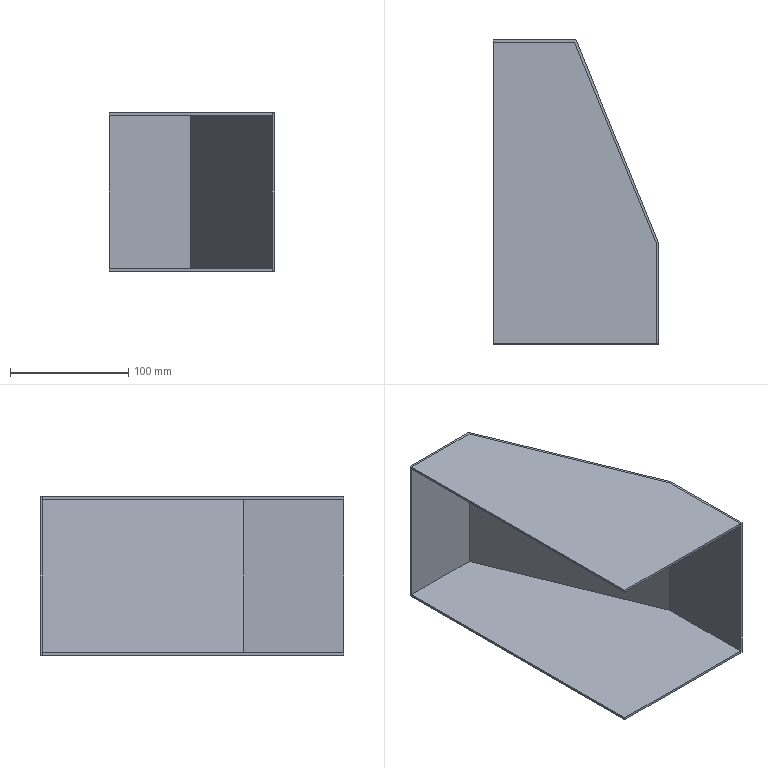Part | SolidWorks | features ICE 2, ExtruThin 1, WeldmentFeature 1 | 3 solids | 24 faces | box 140 x 257 x 134 mm | volume 207970 mm3 | plane 24
STEP:
#1=CARTESIAN_POINT('',(138.,-172.391,0.));
#2=VERTEX_POINT('',#1);
#3=CARTESIAN_POINT('',(138.,-257.,0.));
#4=VERTEX_POINT('',#3);
#5=CARTESIAN_POINT('',(138.,-172.,0.));
#6=DIRECTION('',(0.,-1.,0.));
#7=VECTOR('',#6,1000.);
#8=LINE('',#5,#7);
#9=EDGE_CURVE('',#2,#4,#8,.T.);
#10=ORIENTED_EDGE('',*,*,#9,.T.);
#11=CARTESIAN_POINT('',(138.,-257.,134.));
#12=VERTEX_POINT('',#11);
#13=CARTESIAN_POINT('',(138.,-257.,134.));
#14=DIRECTION('',(0.,0.,-1.));
#15=VECTOR('',#14,1000.);
#16=LINE('',#13,#15);
#17=EDGE_CURVE('',#12,#4,#16,.T.);
#18=ORIENTED_EDGE('',*,*,#17,.F.);
#19=CARTESIAN_POINT('',(138.,-172.391,134.));
#20=VERTEX_POINT('',#19);
#21=CARTESIAN_POINT('',(138.,-172.,134.));
#22=DIRECTION('',(0.,-1.,0.));
#23=VECTOR('',#22,1000.);
#24=LINE('',#21,#23);
#25=EDGE_CURVE('',#20,#12,#24,.T.);
#26=ORIENTED_EDGE('',*,*,#25,.F.);
#27=CARTESIAN_POINT('',(138.,-172.391,134.));
#28=DIRECTION('',(0.,0.,-1.));
#29=VECTOR('',#28,1000.);
#30=LINE('',#27,#29);
#31=EDGE_CURVE('',#20,#2,#30,.T.);
#32=ORIENTED_EDGE('',*,*,#31,.T.);
#33=EDGE_LOOP('',(#10,#18,#26,#32));
#34=FACE_OUTER_BOUND('',#33,.T.);
#35=CARTESIAN_POINT('',(138.,-172.,134.));
#36=DIRECTION('',(1.,0.,0.));
#37=DIRECTION('',(0.,1.,0.));
#38=AXIS2_PLACEMENT_3D('',#35,#36,#37);
#39=PLANE('',#38);
#40=ADVANCED_FACE('',(#34),#39,.F.);
#41=CARTESIAN_POINT('',(140.,-257.,0.));
#42=VERTEX_POINT('',#41);
#43=CARTESIAN_POINT('',(140.,-257.,0.));
#44=DIRECTION('',(-1.,0.,0.));
#45=VECTOR('',#44,1000.);
#46=LINE('',#43,#45);
#47=EDGE_CURVE('',#42,#4,#46,.T.);
#48=ORIENTED_EDGE('',*,*,#47,.F.);
#49=CARTESIAN_POINT('',(140.,-257.,134.));
#50=VERTEX_POINT('',#49);
#51=CARTESIAN_POINT('',(140.,-257.,134.));
#52=DIRECTION('',(0.,0.,-1.));
#53=VECTOR('',#52,1000.);
#54=LINE('',#51,#53);
#55=EDGE_CURVE('',#50,#42,#54,.T.);
#56=ORIENTED_EDGE('',*,*,#55,.F.);
#57=CARTESIAN_POINT('',(140.,-257.,134.));
#58=DIRECTION('',(-1.,0.,0.));
#59=VECTOR('',#58,1000.);
#60=LINE('',#57,#59);
#61=EDGE_CURVE('',#50,#12,#60,.T.);
#62=ORIENTED_EDGE('',*,*,#61,.T.);
#63=ORIENTED_EDGE('',*,*,#17,.T.);
#64=EDGE_LOOP('',(#48,#56,#62,#63));
#65=FACE_OUTER_BOUND('',#64,.T.);
#66=CARTESIAN_POINT('',(140.,-257.,134.));
#67=DIRECTION('',(0.,-1.,0.));
#68=DIRECTION('',(0.,0.,-1.));
#69=AXIS2_PLACEMENT_3D('',#66,#67,#68);
#70=PLANE('',#69);
#71=ADVANCED_FACE('',(#65),#70,.T.);
#72=CARTESIAN_POINT('',(140.,-172.,0.));
#73=VERTEX_POINT('',#72);
#74=CARTESIAN_POINT('',(140.,-172.,0.));
#75=DIRECTION('',(0.,-1.,0.));
#76=VECTOR('',#75,1000.);
#77=LINE('',#74,#76);
#78=EDGE_CURVE('',#73,#42,#77,.T.);
#79=ORIENTED_EDGE('',*,*,#78,.F.);
#80=CARTESIAN_POINT('',(140.,-172.,134.));
#81=VERTEX_POINT('',#80);
#82=CARTESIAN_POINT('',(140.,-172.,134.));
#83=DIRECTION('',(0.,0.,-1.));
#84=VECTOR('',#83,1000.);
#85=LINE('',#82,#84);
#86=EDGE_CURVE('',#81,#73,#85,.T.);
#87=ORIENTED_EDGE('',*,*,#86,.F.);
#88=CARTESIAN_POINT('',(140.,-172.,134.));
#89=DIRECTION('',(0.,-1.,0.));
#90=VECTOR('',#89,1000.);
#91=LINE('',#88,#90);
#92=EDGE_CURVE('',#81,#50,#91,.T.);
#93=ORIENTED_EDGE('',*,*,#92,.T.);
#94=ORIENTED_EDGE('',*,*,#55,.T.);
#95=EDGE_LOOP('',(#79,#87,#93,#94));
#96=FACE_OUTER_BOUND('',#95,.T.);
#97=CARTESIAN_POINT('',(140.,-172.,134.));
#98=DIRECTION('',(1.,0.,0.));
#99=DIRECTION('',(0.,1.,0.));
#100=AXIS2_PLACEMENT_3D('',#97,#98,#99);
#101=PLANE('',#100);
#102=ADVANCED_FACE('',(#96),#101,.T.);
#103=CARTESIAN_POINT('',(70.,0.,0.));
#104=VERTEX_POINT('',#103);
#105=CARTESIAN_POINT('',(70.,0.,0.));
#106=DIRECTION('',(0.377,-0.9262,0.));
#107=VECTOR('',#106,1000.);
#108=LINE('',#105,#107);
#109=EDGE_CURVE('',#104,#73,#108,.T.);
#110=ORIENTED_EDGE('',*,*,#109,.F.);
#111=CARTESIAN_POINT('',(70.,0.,134.));
#112=VERTEX_POINT('',#111);
#113=CARTESIAN_POINT('',(70.,0.,134.));
#114=DIRECTION('',(0.,0.,-1.));
#115=VECTOR('',#114,1000.);
#116=LINE('',#113,#115);
#117=EDGE_CURVE('',#112,#104,#116,.T.);
#118=ORIENTED_EDGE('',*,*,#117,.F.);
#119=CARTESIAN_POINT('',(70.,0.,134.));
#120=DIRECTION('',(0.377,-0.9262,0.));
#121=VECTOR('',#120,1000.);
#122=LINE('',#119,#121);
#123=EDGE_CURVE('',#112,#81,#122,.T.);
#124=ORIENTED_EDGE('',*,*,#123,.T.);
#125=ORIENTED_EDGE('',*,*,#86,.T.);
#126=EDGE_LOOP('',(#110,#118,#124,#125));
#127=FACE_OUTER_BOUND('',#126,.T.);
#128=CARTESIAN_POINT('',(70.,0.,134.));
#129=DIRECTION('',(0.9262,0.377,0.));
#130=DIRECTION('',(-0.377,0.9262,0.));
#131=AXIS2_PLACEMENT_3D('',#128,#129,#130);
#132=PLANE('',#131);
#133=ADVANCED_FACE('',(#127),#132,.T.);
#134=CARTESIAN_POINT('',(0.,0.,0.));
#135=VERTEX_POINT('',#134);
#136=CARTESIAN_POINT('',(0.,0.,0.));
#137=DIRECTION('',(1.,0.,0.));
#138=VECTOR('',#137,1000.);
#139=LINE('',#136,#138);
#140=EDGE_CURVE('',#135,#104,#139,.T.);
#141=ORIENTED_EDGE('',*,*,#140,.F.);
#142=CARTESIAN_POINT('',(0.,0.,134.));
#143=VERTEX_POINT('',#142);
#144=CARTESIAN_POINT('',(0.,0.,134.));
#145=DIRECTION('',(0.,0.,-1.));
#146=VECTOR('',#145,1000.);
#147=LINE('',#144,#146);
#148=EDGE_CURVE('',#143,#135,#147,.T.);
#149=ORIENTED_EDGE('',*,*,#148,.F.);
#150=CARTESIAN_POINT('',(0.,0.,134.));
#151=DIRECTION('',(1.,0.,0.));
#152=VECTOR('',#151,1000.);
#153=LINE('',#150,#152);
#154=EDGE_CURVE('',#143,#112,#153,.T.);
#155=ORIENTED_EDGE('',*,*,#154,.T.);
#156=ORIENTED_EDGE('',*,*,#117,.T.);
#157=EDGE_LOOP('',(#141,#149,#155,#156));
#158=FACE_OUTER_BOUND('',#157,.T.);
#159=CARTESIAN_POINT('',(0.,0.,134.));
#160=DIRECTION('',(0.,1.,0.));
#161=DIRECTION('',(0.,0.,1.));
#162=AXIS2_PLACEMENT_3D('',#159,#160,#161);
#163=PLANE('',#162);
#164=ADVANCED_FACE('',(#158),#163,.T.);
#165=CARTESIAN_POINT('',(0.,-2.,0.));
#166=VERTEX_POINT('',#165);
#167=CARTESIAN_POINT('',(0.,-2.,0.));
#168=DIRECTION('',(0.,1.,0.));
#169=VECTOR('',#168,1000.);
#170=LINE('',#167,#169);
#171=EDGE_CURVE('',#166,#135,#170,.T.);
#172=ORIENTED_EDGE('',*,*,#171,.F.);
#173=CARTESIAN_POINT('',(0.,-2.,134.));
#174=VERTEX_POINT('',#173);
#175=CARTESIAN_POINT('',(0.,-2.,134.));
#176=DIRECTION('',(0.,0.,-1.));
#177=VECTOR('',#176,1000.);
#178=LINE('',#175,#177);
#179=EDGE_CURVE('',#174,#166,#178,.T.);
#180=ORIENTED_EDGE('',*,*,#179,.F.);
#181=CARTESIAN_POINT('',(0.,-2.,134.));
#182=DIRECTION('',(0.,1.,0.));
#183=VECTOR('',#182,1000.);
#184=LINE('',#181,#183);
#185=EDGE_CURVE('',#174,#143,#184,.T.);
#186=ORIENTED_EDGE('',*,*,#185,.T.);
#187=ORIENTED_EDGE('',*,*,#148,.T.);
#188=EDGE_LOOP('',(#172,#180,#186,#187));
#189=FACE_OUTER_BOUND('',#188,.T.);
#190=CARTESIAN_POINT('',(0.,-2.,134.));
#191=DIRECTION('',(-1.,0.,0.));
#192=DIRECTION('',(0.,0.,1.));
#193=AXIS2_PLACEMENT_3D('',#190,#191,#192);
#194=PLANE('',#193);
#195=ADVANCED_FACE('',(#189),#194,.T.);
#196=CARTESIAN_POINT('',(68.655,-2.,0.));
#197=VERTEX_POINT('',#196);
#198=CARTESIAN_POINT('',(0.,-2.,0.));
#199=DIRECTION('',(1.,0.,0.));
#200=VECTOR('',#199,1000.);
#201=LINE('',#198,#200);
#202=EDGE_CURVE('',#166,#197,#201,.T.);
#203=ORIENTED_EDGE('',*,*,#202,.T.);
#204=CARTESIAN_POINT('',(68.655,-2.,134.));
#205=VERTEX_POINT('',#204);
#206=CARTESIAN_POINT('',(68.655,-2.,134.));
#207=DIRECTION('',(0.,0.,-1.));
#208=VECTOR('',#207,1000.);
#209=LINE('',#206,#208);
#210=EDGE_CURVE('',#205,#197,#209,.T.);
#211=ORIENTED_EDGE('',*,*,#210,.F.);
#212=CARTESIAN_POINT('',(0.,-2.,134.));
#213=DIRECTION('',(1.,0.,0.));
#214=VECTOR('',#213,1000.);
#215=LINE('',#212,#214);
#216=EDGE_CURVE('',#174,#205,#215,.T.);
#217=ORIENTED_EDGE('',*,*,#216,.F.);
#218=ORIENTED_EDGE('',*,*,#179,.T.);
#219=EDGE_LOOP('',(#203,#211,#217,#218));
#220=FACE_OUTER_BOUND('',#219,.T.);
#221=CARTESIAN_POINT('',(0.,-2.,134.));
#222=DIRECTION('',(0.,1.,0.));
#223=DIRECTION('',(0.,0.,1.));
#224=AXIS2_PLACEMENT_3D('',#221,#222,#223);
#225=PLANE('',#224);
#226=ADVANCED_FACE('',(#220),#225,.F.);
#227=CARTESIAN_POINT('',(68.148,-0.7539,0.));
#228=DIRECTION('',(0.377,-0.9262,0.));
#229=VECTOR('',#228,1000.);
#230=LINE('',#227,#229);
#231=EDGE_CURVE('',#197,#2,#230,.T.);
#232=ORIENTED_EDGE('',*,*,#231,.T.);
#233=ORIENTED_EDGE('',*,*,#31,.F.);
#234=CARTESIAN_POINT('',(68.148,-0.7539,134.));
#235=DIRECTION('',(0.377,-0.9262,0.));
#236=VECTOR('',#235,1000.);
#237=LINE('',#234,#236);
#238=EDGE_CURVE('',#205,#20,#237,.T.);
#239=ORIENTED_EDGE('',*,*,#238,.F.);
#240=ORIENTED_EDGE('',*,*,#210,.T.);
#241=EDGE_LOOP('',(#232,#233,#239,#240));
#242=FACE_OUTER_BOUND('',#241,.T.);
#243=CARTESIAN_POINT('',(68.148,-0.7539,134.));
#244=DIRECTION('',(0.9262,0.377,0.));
#245=DIRECTION('',(-0.377,0.9262,0.));
#246=AXIS2_PLACEMENT_3D('',#243,#244,#245);
#247=PLANE('',#246);
#248=ADVANCED_FACE('',(#242),#247,.F.);
#249=ORIENTED_EDGE('',*,*,#25,.T.);
#250=ORIENTED_EDGE('',*,*,#61,.F.);
#251=ORIENTED_EDGE('',*,*,#92,.F.);
#252=ORIENTED_EDGE('',*,*,#123,.F.);
#253=ORIENTED_EDGE('',*,*,#154,.F.);
#254=ORIENTED_EDGE('',*,*,#185,.F.);
#255=ORIENTED_EDGE('',*,*,#216,.T.);
#256=ORIENTED_EDGE('',*,*,#238,.T.);
#257=EDGE_LOOP('',(#249,#250,#251,#252,#253,#254,#255,#256));
#258=FACE_OUTER_BOUND('',#257,.T.);
#259=CARTESIAN_POINT('',(0.,0.,134.));
#260=DIRECTION('',(0.,0.,-1.));
#261=DIRECTION('',(-1.,0.,0.));
#262=AXIS2_PLACEMENT_3D('',#259,#260,#261);
#263=PLANE('',#262);
#264=ADVANCED_FACE('',(#258),#263,.F.);
#265=ORIENTED_EDGE('',*,*,#9,.F.);
#266=ORIENTED_EDGE('',*,*,#231,.F.);
#267=ORIENTED_EDGE('',*,*,#202,.F.);
#268=ORIENTED_EDGE('',*,*,#171,.T.);
#269=ORIENTED_EDGE('',*,*,#140,.T.);
#270=ORIENTED_EDGE('',*,*,#109,.T.);
#271=ORIENTED_EDGE('',*,*,#78,.T.);
#272=ORIENTED_EDGE('',*,*,#47,.T.);
#273=EDGE_LOOP('',(#265,#266,#267,#268,#269,#270,#271,#272));
#274=FACE_OUTER_BOUND('',#273,.T.);
#275=CARTESIAN_POINT('',(0.,0.,0.));
#276=DIRECTION('',(0.,0.,-1.));
#277=DIRECTION('',(-1.,0.,0.));
#278=AXIS2_PLACEMENT_3D('',#275,#276,#277);
#279=PLANE('',#278);
#280=ADVANCED_FACE('',(#274),#279,.T.);
#281=CLOSED_SHELL('',(#40,#71,#102,#133,#164,#195,#226,#248,#264,#280));
#282=MANIFOLD_SOLID_BREP('',#281);
#283=CARTESIAN_POINT('',(0.,-2.,134.));
#284=VERTEX_POINT('',#283);
#285=CARTESIAN_POINT('',(0.,-257.,134.));
#286=VERTEX_POINT('',#285);
#287=CARTESIAN_POINT('',(0.,-257.,134.));
#288=DIRECTION('',(0.,-1.,0.));
#289=VECTOR('',#288,1000.);
#290=LINE('',#287,#289);
#291=EDGE_CURVE('',#284,#286,#290,.T.);
#292=ORIENTED_EDGE('',*,*,#291,.F.);
#293=CARTESIAN_POINT('',(0.,-2.,132.));
#294=VERTEX_POINT('',#293);
#295=CARTESIAN_POINT('',(0.,-2.,132.));
#296=DIRECTION('',(0.,0.,1.));
#297=VECTOR('',#296,1000.);
#298=LINE('',#295,#297);
#299=EDGE_CURVE('',#294,#284,#298,.T.);
#300=ORIENTED_EDGE('',*,*,#299,.F.);
#301=CARTESIAN_POINT('',(0.,-257.,132.));
#302=VERTEX_POINT('',#301);
#303=CARTESIAN_POINT('',(0.,-257.,132.));
#304=DIRECTION('',(0.,-1.,0.));
#305=VECTOR('',#304,1000.);
#306=LINE('',#303,#305);
#307=EDGE_CURVE('',#294,#302,#306,.T.);
#308=ORIENTED_EDGE('',*,*,#307,.T.);
#309=CARTESIAN_POINT('',(0.,-257.,132.));
#310=DIRECTION('',(0.,0.,1.));
#311=VECTOR('',#310,1000.);
#312=LINE('',#309,#311);
#313=EDGE_CURVE('',#302,#286,#312,.T.);
#314=ORIENTED_EDGE('',*,*,#313,.T.);
#315=EDGE_LOOP('',(#292,#300,#308,#314));
#316=FACE_OUTER_BOUND('',#315,.T.);
#317=CARTESIAN_POINT('',(0.,-257.,132.));
#318=DIRECTION('',(-1.,0.,0.));
#319=DIRECTION('',(0.,0.,1.));
#320=AXIS2_PLACEMENT_3D('',#317,#318,#319);
#321=PLANE('',#320);
#322=ADVANCED_FACE('',(#316),#321,.T.);
#323=CARTESIAN_POINT('',(68.655,-2.,134.));
#324=VERTEX_POINT('',#323);
#325=CARTESIAN_POINT('',(0.,-2.,134.));
#326=DIRECTION('',(-1.,0.,0.));
#327=VECTOR('',#326,1000.);
#328=LINE('',#325,#327);
#329=EDGE_CURVE('',#324,#284,#328,.T.);
#330=ORIENTED_EDGE('',*,*,#329,.F.);
#331=CARTESIAN_POINT('',(68.655,-2.,132.));
#332=VERTEX_POINT('',#331);
#333=CARTESIAN_POINT('',(68.655,-2.,132.));
#334=DIRECTION('',(0.,0.,1.));
#335=VECTOR('',#334,1000.);
#336=LINE('',#333,#335);
#337=EDGE_CURVE('',#332,#324,#336,.T.);
#338=ORIENTED_EDGE('',*,*,#337,.F.);
#339=CARTESIAN_POINT('',(0.,-2.,132.));
#340=DIRECTION('',(-1.,0.,0.));
#341=VECTOR('',#340,1000.);
#342=LINE('',#339,#341);
#343=EDGE_CURVE('',#332,#294,#342,.T.);
#344=ORIENTED_EDGE('',*,*,#343,.T.);
#345=ORIENTED_EDGE('',*,*,#299,.T.);
#346=EDGE_LOOP('',(#330,#338,#344,#345));
#347=FACE_OUTER_BOUND('',#346,.T.);
#348=CARTESIAN_POINT('',(0.,-2.,132.));
#349=DIRECTION('',(0.,1.,0.));
#350=DIRECTION('',(-1.,0.,0.));
#351=AXIS2_PLACEMENT_3D('',#348,#349,#350);
#352=PLANE('',#351);
#353=ADVANCED_FACE('',(#347),#352,.T.);
#354=CARTESIAN_POINT('',(138.,-172.391,134.));
#355=VERTEX_POINT('',#354);
#356=CARTESIAN_POINT('',(68.655,-2.,134.));
#357=DIRECTION('',(-0.377,0.9262,0.));
#358=VECTOR('',#357,1000.);
#359=LINE('',#356,#358);
#360=EDGE_CURVE('',#355,#324,#359,.T.);
#361=ORIENTED_EDGE('',*,*,#360,.F.);
#362=CARTESIAN_POINT('',(138.,-172.391,132.));
#363=VERTEX_POINT('',#362);
#364=CARTESIAN_POINT('',(138.,-172.391,132.));
#365=DIRECTION('',(0.,0.,1.));
#366=VECTOR('',#365,1000.);
#367=LINE('',#364,#366);
#368=EDGE_CURVE('',#363,#355,#367,.T.);
#369=ORIENTED_EDGE('',*,*,#368,.F.);
#370=CARTESIAN_POINT('',(68.655,-2.,132.));
#371=DIRECTION('',(-0.377,0.9262,0.));
#372=VECTOR('',#371,1000.);
#373=LINE('',#370,#372);
#374=EDGE_CURVE('',#363,#332,#373,.T.);
#375=ORIENTED_EDGE('',*,*,#374,.T.);
#376=ORIENTED_EDGE('',*,*,#337,.T.);
#377=EDGE_LOOP('',(#361,#369,#375,#376));
#378=FACE_OUTER_BOUND('',#377,.T.);
#379=CARTESIAN_POINT('',(68.655,-2.,132.));
#380=DIRECTION('',(0.9262,0.377,0.));
#381=DIRECTION('',(-0.377,0.9262,0.));
#382=AXIS2_PLACEMENT_3D('',#379,#380,#381);
#383=PLANE('',#382);
#384=ADVANCED_FACE('',(#378),#383,.T.);
#385=CARTESIAN_POINT('',(138.,-257.,134.));
#386=VERTEX_POINT('',#385);
#387=CARTESIAN_POINT('',(138.,-172.391,134.));
#388=DIRECTION('',(0.,1.,0.));
#389=VECTOR('',#388,1000.);
#390=LINE('',#387,#389);
#391=EDGE_CURVE('',#386,#355,#390,.T.);
#392=ORIENTED_EDGE('',*,*,#391,.F.);
#393=CARTESIAN_POINT('',(138.,-257.,132.));
#394=VERTEX_POINT('',#393);
#395=CARTESIAN_POINT('',(138.,-257.,132.));
#396=DIRECTION('',(0.,0.,1.));
#397=VECTOR('',#396,1000.);
#398=LINE('',#395,#397);
#399=EDGE_CURVE('',#394,#386,#398,.T.);
#400=ORIENTED_EDGE('',*,*,#399,.F.);
#401=CARTESIAN_POINT('',(138.,-172.391,132.));
#402=DIRECTION('',(0.,1.,0.));
#403=VECTOR('',#402,1000.);
#404=LINE('',#401,#403);
#405=EDGE_CURVE('',#394,#363,#404,.T.);
#406=ORIENTED_EDGE('',*,*,#405,.T.);
#407=ORIENTED_EDGE('',*,*,#368,.T.);
#408=EDGE_LOOP('',(#392,#400,#406,#407));
#409=FACE_OUTER_BOUND('',#408,.T.);
#410=CARTESIAN_POINT('',(138.,-172.391,132.));
#411=DIRECTION('',(1.,0.,0.));
#412=DIRECTION('',(0.,1.,0.));
#413=AXIS2_PLACEMENT_3D('',#410,#411,#412);
#414=PLANE('',#413);
#415=ADVANCED_FACE('',(#409),#414,.T.);
#416=CARTESIAN_POINT('',(138.,-257.,134.));
#417=DIRECTION('',(1.,0.,0.));
#418=VECTOR('',#417,1000.);
#419=LINE('',#416,#418);
#420=EDGE_CURVE('',#286,#386,#419,.T.);
#421=ORIENTED_EDGE('',*,*,#420,.F.);
#422=ORIENTED_EDGE('',*,*,#313,.F.);
#423=CARTESIAN_POINT('',(138.,-257.,132.));
#424=DIRECTION('',(1.,0.,0.));
#425=VECTOR('',#424,1000.);
#426=LINE('',#423,#425);
#427=EDGE_CURVE('',#302,#394,#426,.T.);
#428=ORIENTED_EDGE('',*,*,#427,.T.);
#429=ORIENTED_EDGE('',*,*,#399,.T.);
#430=EDGE_LOOP('',(#421,#422,#428,#429));
#431=FACE_OUTER_BOUND('',#430,.T.);
#432=CARTESIAN_POINT('',(138.,-257.,132.));
#433=DIRECTION('',(0.,-1.,0.));
#434=DIRECTION('',(0.,0.,-1.));
#435=AXIS2_PLACEMENT_3D('',#432,#433,#434);
#436=PLANE('',#435);
#437=ADVANCED_FACE('',(#431),#436,.T.);
#438=ORIENTED_EDGE('',*,*,#307,.F.);
#439=ORIENTED_EDGE('',*,*,#343,.F.);
#440=ORIENTED_EDGE('',*,*,#374,.F.);
#441=ORIENTED_EDGE('',*,*,#405,.F.);
#442=ORIENTED_EDGE('',*,*,#427,.F.);
#443=EDGE_LOOP('',(#438,#439,#440,#441,#442));
#444=FACE_OUTER_BOUND('',#443,.T.);
#445=CARTESIAN_POINT('',(0.,0.,132.));
#446=DIRECTION('',(0.,0.,-1.));
#447=DIRECTION('',(-1.,0.,0.));
#448=AXIS2_PLACEMENT_3D('',#445,#446,#447);
#449=PLANE('',#448);
#450=ADVANCED_FACE('',(#444),#449,.T.);
#451=ORIENTED_EDGE('',*,*,#291,.T.);
#452=ORIENTED_EDGE('',*,*,#420,.T.);
#453=ORIENTED_EDGE('',*,*,#391,.T.);
#454=ORIENTED_EDGE('',*,*,#360,.T.);
#455=ORIENTED_EDGE('',*,*,#329,.T.);
#456=EDGE_LOOP('',(#451,#452,#453,#454,#455));
#457=FACE_OUTER_BOUND('',#456,.T.);
#458=CARTESIAN_POINT('',(0.,0.,134.));
#459=DIRECTION('',(0.,0.,-1.));
#460=DIRECTION('',(-1.,0.,0.));
#461=AXIS2_PLACEMENT_3D('',#458,#459,#460);
#462=PLANE('',#461);
#463=ADVANCED_FACE('',(#457),#462,.F.);
#464=CLOSED_SHELL('',(#322,#353,#384,#415,#437,#450,#463));
#465=MANIFOLD_SOLID_BREP('',#464);
#466=CARTESIAN_POINT('',(68.655,-2.,0.));
#467=VERTEX_POINT('',#466);
#468=CARTESIAN_POINT('',(138.,-172.391,0.));
#469=VERTEX_POINT('',#468);
#470=CARTESIAN_POINT('',(58.201,23.686,0.));
#471=DIRECTION('',(0.377,-0.9262,0.));
#472=VECTOR('',#471,1000.);
#473=LINE('',#470,#472);
#474=EDGE_CURVE('',#467,#469,#473,.T.);
#475=ORIENTED_EDGE('',*,*,#474,.F.);
#476=CARTESIAN_POINT('',(68.655,-2.,2.));
#477=VERTEX_POINT('',#476);
#478=CARTESIAN_POINT('',(68.655,-2.,2.));
#479=DIRECTION('',(0.,0.,-1.));
#480=VECTOR('',#479,1000.);
#481=LINE('',#478,#480);
#482=EDGE_CURVE('',#477,#467,#481,.T.);
#483=ORIENTED_EDGE('',*,*,#482,.F.);
#484=CARTESIAN_POINT('',(138.,-172.391,2.));
#485=VERTEX_POINT('',#484);
#486=CARTESIAN_POINT('',(58.201,23.686,2.));
#487=DIRECTION('',(0.377,-0.9262,0.));
#488=VECTOR('',#487,1000.);
#489=LINE('',#486,#488);
#490=EDGE_CURVE('',#477,#485,#489,.T.);
#491=ORIENTED_EDGE('',*,*,#490,.T.);
#492=CARTESIAN_POINT('',(138.,-172.391,2.));
#493=DIRECTION('',(0.,0.,-1.));
#494=VECTOR('',#493,1000.);
#495=LINE('',#492,#494);
#496=EDGE_CURVE('',#485,#469,#495,.T.);
#497=ORIENTED_EDGE('',*,*,#496,.T.);
#498=EDGE_LOOP('',(#475,#483,#491,#497));
#499=FACE_OUTER_BOUND('',#498,.T.);
#500=CARTESIAN_POINT('',(58.201,23.686,2.));
#501=DIRECTION('',(0.9262,0.377,0.));
#502=DIRECTION('',(-0.377,0.9262,0.));
#503=AXIS2_PLACEMENT_3D('',#500,#501,#502);
#504=PLANE('',#503);
#505=ADVANCED_FACE('',(#499),#504,.T.);
#506=CARTESIAN_POINT('',(0.,-2.,0.));
#507=VERTEX_POINT('',#506);
#508=CARTESIAN_POINT('',(0.,-2.,0.));
#509=DIRECTION('',(1.,0.,0.));
#510=VECTOR('',#509,1000.);
#511=LINE('',#508,#510);
#512=EDGE_CURVE('',#507,#467,#511,.T.);
#513=ORIENTED_EDGE('',*,*,#512,.F.);
#514=CARTESIAN_POINT('',(0.,-2.,2.));
#515=VERTEX_POINT('',#514);
#516=CARTESIAN_POINT('',(0.,-2.,2.));
#517=DIRECTION('',(0.,0.,-1.));
#518=VECTOR('',#517,1000.);
#519=LINE('',#516,#518);
#520=EDGE_CURVE('',#515,#507,#519,.T.);
#521=ORIENTED_EDGE('',*,*,#520,.F.);
#522=CARTESIAN_POINT('',(0.,-2.,2.));
#523=DIRECTION('',(1.,0.,0.));
#524=VECTOR('',#523,1000.);
#525=LINE('',#522,#524);
#526=EDGE_CURVE('',#515,#477,#525,.T.);
#527=ORIENTED_EDGE('',*,*,#526,.T.);
#528=ORIENTED_EDGE('',*,*,#482,.T.);
#529=EDGE_LOOP('',(#513,#521,#527,#528));
#530=FACE_OUTER_BOUND('',#529,.T.);
#531=CARTESIAN_POINT('',(0.,-2.,2.));
#532=DIRECTION('',(0.,1.,0.));
#533=DIRECTION('',(-1.,0.,0.));
#534=AXIS2_PLACEMENT_3D('',#531,#532,#533);
#535=PLANE('',#534);
#536=ADVANCED_FACE('',(#530),#535,.T.);
#537=CARTESIAN_POINT('',(0.,-257.,0.));
#538=VERTEX_POINT('',#537);
#539=CARTESIAN_POINT('',(0.,0.,0.));
#540=DIRECTION('',(0.,1.,0.));
#541=VECTOR('',#540,1000.);
#542=LINE('',#539,#541);
#543=EDGE_CURVE('',#538,#507,#542,.T.);
#544=ORIENTED_EDGE('',*,*,#543,.F.);
#545=CARTESIAN_POINT('',(0.,-257.,2.));
#546=VERTEX_POINT('',#545);
#547=CARTESIAN_POINT('',(0.,-257.,2.));
#548=DIRECTION('',(0.,0.,-1.));
#549=VECTOR('',#548,1000.);
#550=LINE('',#547,#549);
#551=EDGE_CURVE('',#546,#538,#550,.T.);
#552=ORIENTED_EDGE('',*,*,#551,.F.);
#553=CARTESIAN_POINT('',(0.,0.,2.));
#554=DIRECTION('',(0.,1.,0.));
#555=VECTOR('',#554,1000.);
#556=LINE('',#553,#555);
#557=EDGE_CURVE('',#546,#515,#556,.T.);
#558=ORIENTED_EDGE('',*,*,#557,.T.);
#559=ORIENTED_EDGE('',*,*,#520,.T.);
#560=EDGE_LOOP('',(#544,#552,#558,#559));
#561=FACE_OUTER_BOUND('',#560,.T.);
#562=CARTESIAN_POINT('',(0.,0.,2.));
#563=DIRECTION('',(-1.,0.,0.));
#564=DIRECTION('',(0.,0.,1.));
#565=AXIS2_PLACEMENT_3D('',#562,#563,#564);
#566=PLANE('',#565);
#567=ADVANCED_FACE('',(#561),#566,.T.);
#568=CARTESIAN_POINT('',(138.,-257.,0.));
#569=VERTEX_POINT('',#568);
#570=CARTESIAN_POINT('',(0.,-257.,0.));
#571=DIRECTION('',(-1.,0.,0.));
#572=VECTOR('',#571,1000.);
#573=LINE('',#570,#572);
#574=EDGE_CURVE('',#569,#538,#573,.T.);
#575=ORIENTED_EDGE('',*,*,#574,.F.);
#576=CARTESIAN_POINT('',(138.,-257.,2.));
#577=VERTEX_POINT('',#576);
#578=CARTESIAN_POINT('',(138.,-257.,2.));
#579=DIRECTION('',(0.,0.,-1.));
#580=VECTOR('',#579,1000.);
#581=LINE('',#578,#580);
#582=EDGE_CURVE('',#577,#569,#581,.T.);
#583=ORIENTED_EDGE('',*,*,#582,.F.);
#584=CARTESIAN_POINT('',(0.,-257.,2.));
#585=DIRECTION('',(-1.,0.,0.));
#586=VECTOR('',#585,1000.);
#587=LINE('',#584,#586);
#588=EDGE_CURVE('',#577,#546,#587,.T.);
#589=ORIENTED_EDGE('',*,*,#588,.T.);
#590=ORIENTED_EDGE('',*,*,#551,.T.);
#591=EDGE_LOOP('',(#575,#583,#589,#590));
#592=FACE_OUTER_BOUND('',#591,.T.);
#593=CARTESIAN_POINT('',(0.,-257.,2.));
#594=DIRECTION('',(0.,-1.,0.));
#595=DIRECTION('',(0.,0.,-1.));
#596=AXIS2_PLACEMENT_3D('',#593,#594,#595);
#597=PLANE('',#596);
#598=ADVANCED_FACE('',(#592),#597,.T.);
#599=CARTESIAN_POINT('',(138.,0.,0.));
#600=DIRECTION('',(0.,-1.,0.));
#601=VECTOR('',#600,1000.);
#602=LINE('',#599,#601);
#603=EDGE_CURVE('',#469,#569,#602,.T.);
#604=ORIENTED_EDGE('',*,*,#603,.F.);
#605=ORIENTED_EDGE('',*,*,#496,.F.);
#606=CARTESIAN_POINT('',(138.,0.,2.));
#607=DIRECTION('',(0.,-1.,0.));
#608=VECTOR('',#607,1000.);
#609=LINE('',#606,#608);
#610=EDGE_CURVE('',#485,#577,#609,.T.);
#611=ORIENTED_EDGE('',*,*,#610,.T.);
#612=ORIENTED_EDGE('',*,*,#582,.T.);
#613=EDGE_LOOP('',(#604,#605,#611,#612));
#614=FACE_OUTER_BOUND('',#613,.T.);
#615=CARTESIAN_POINT('',(138.,0.,2.));
#616=DIRECTION('',(1.,0.,0.));
#617=DIRECTION('',(0.,1.,0.));
#618=AXIS2_PLACEMENT_3D('',#615,#616,#617);
#619=PLANE('',#618);
#620=ADVANCED_FACE('',(#614),#619,.T.);
#621=ORIENTED_EDGE('',*,*,#490,.F.);
#622=ORIENTED_EDGE('',*,*,#526,.F.);
#623=ORIENTED_EDGE('',*,*,#557,.F.);
#624=ORIENTED_EDGE('',*,*,#588,.F.);
#625=ORIENTED_EDGE('',*,*,#610,.F.);
#626=EDGE_LOOP('',(#621,#622,#623,#624,#625));
#627=FACE_OUTER_BOUND('',#626,.T.);
#628=CARTESIAN_POINT('',(0.,0.,2.));
#629=DIRECTION('',(0.,0.,-1.));
#630=DIRECTION('',(-1.,0.,0.));
#631=AXIS2_PLACEMENT_3D('',#628,#629,#630);
#632=PLANE('',#631);
#633=ADVANCED_FACE('',(#627),#632,.F.);
#634=ORIENTED_EDGE('',*,*,#474,.T.);
#635=ORIENTED_EDGE('',*,*,#603,.T.);
#636=ORIENTED_EDGE('',*,*,#574,.T.);
#637=ORIENTED_EDGE('',*,*,#543,.T.);
#638=ORIENTED_EDGE('',*,*,#512,.T.);
#639=EDGE_LOOP('',(#634,#635,#636,#637,#638));
#640=FACE_OUTER_BOUND('',#639,.T.);
#641=CARTESIAN_POINT('',(0.,0.,0.));
#642=DIRECTION('',(0.,0.,-1.));
#643=DIRECTION('',(-1.,0.,0.));
#644=AXIS2_PLACEMENT_3D('',#641,#642,#643);
#645=PLANE('',#644);
#646=ADVANCED_FACE('',(#640),#645,.T.);
#647=CLOSED_SHELL('',(#505,#536,#567,#598,#620,#633,#646));
#648=MANIFOLD_SOLID_BREP('',#647);
#649=CARTESIAN_POINT('',(0.,0.,0.));
#650=DIRECTION('',(0.,0.,1.));
#651=DIRECTION('',(1.,0.,0.));
#652=AXIS2_PLACEMENT_3D('',#649,#650,#651);
#653=(LENGTH_UNIT()NAMED_UNIT(*)SI_UNIT(.MILLI.,.METRE.));
#654=UNCERTAINTY_MEASURE_WITH_UNIT(LENGTH_MEASURE(0.00001),#653,'','');
#655=(NAMED_UNIT(*)PLANE_ANGLE_UNIT()SI_UNIT($,.RADIAN.));
#656=(NAMED_UNIT(*)SI_UNIT($,.STERADIAN.)SOLID_ANGLE_UNIT());
#657=(GEOMETRIC_REPRESENTATION_CONTEXT(3)GLOBAL_UNCERTAINTY_ASSIGNED_CONTEXT((#654))GLOBAL_UNIT_ASSIGNED_CONTEXT((#653,#655,#656))REPRESENTATION_CONTEXT('',''));
#658=ADVANCED_BREP_SHAPE_REPRESENTATION('',(#282,#465,#648,#652),#657);